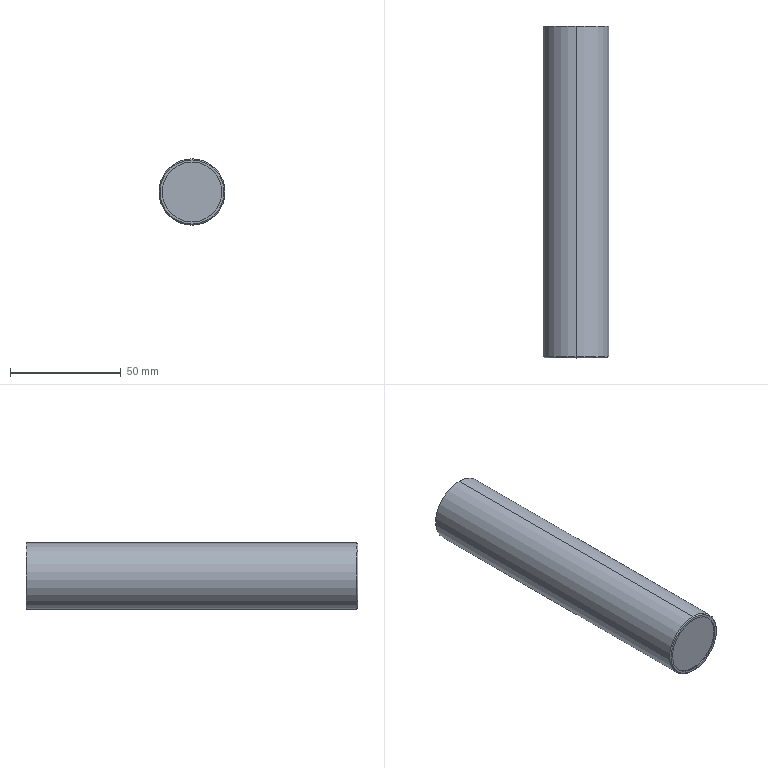Part | SolidWorks | features Chamfer 1, Extrusion 1, RevCut 1 | 1 solid | 12 faces | box 30 x 150 x 30 mm | volume 21279 mm3 | cylinder 6 | plane 4 | cone 2 | commonest cylinder face diameters 27 x4 30 x2
STEP:
#1=CARTESIAN_POINT('',(0.,0.,-14.5));
#2=VERTEX_POINT('',#1);
#3=CARTESIAN_POINT('',(0.,0.,14.5));
#4=VERTEX_POINT('',#3);
#5=CARTESIAN_POINT('',(0.,0.,0.));
#6=DIRECTION('',(0.,-1.,0.));
#7=DIRECTION('',(0.,0.,1.));
#8=AXIS2_PLACEMENT_3D('',#5,#6,#7);
#9=CIRCLE('',#8,14.5);
#10=EDGE_CURVE('',#2,#4,#9,.T.);
#11=ORIENTED_EDGE('',*,*,#10,.F.);
#12=CARTESIAN_POINT('',(0.,0.5,-15.));
#13=VERTEX_POINT('',#12);
#14=CARTESIAN_POINT('',(0.,0.5,-15.));
#15=DIRECTION('',(0.,0.7071,-0.7071));
#16=VECTOR('',#15,1000.);
#17=LINE('',#14,#16);
#18=EDGE_CURVE('',#2,#13,#17,.T.);
#19=ORIENTED_EDGE('',*,*,#18,.T.);
#20=CARTESIAN_POINT('',(0.,0.5,15.));
#21=VERTEX_POINT('',#20);
#22=CARTESIAN_POINT('',(0.,0.5,0.));
#23=DIRECTION('',(0.,1.,0.));
#24=DIRECTION('',(0.,0.,1.));
#25=AXIS2_PLACEMENT_3D('',#22,#23,#24);
#26=CIRCLE('',#25,15.);
#27=EDGE_CURVE('',#21,#13,#26,.T.);
#28=ORIENTED_EDGE('',*,*,#27,.F.);
#29=CARTESIAN_POINT('',(0.,0.5,15.));
#30=DIRECTION('',(0.,0.7071,0.7071));
#31=VECTOR('',#30,1000.);
#32=LINE('',#29,#31);
#33=EDGE_CURVE('',#4,#21,#32,.T.);
#34=ORIENTED_EDGE('',*,*,#33,.F.);
#35=EDGE_LOOP('',(#11,#19,#28,#34));
#36=FACE_OUTER_BOUND('',#35,.T.);
#37=CARTESIAN_POINT('',(0.,0.5,0.));
#38=DIRECTION('',(0.,1.,0.));
#39=DIRECTION('',(0.,0.,1.));
#40=AXIS2_PLACEMENT_3D('',#37,#38,#39);
#41=CONICAL_SURFACE('',#40,15.,0.7854);
#42=ADVANCED_FACE('',(#36),#41,.T.);
#43=CARTESIAN_POINT('',(0.,0.5,13.5));
#44=VERTEX_POINT('',#43);
#45=CARTESIAN_POINT('',(0.,0.5,-13.5));
#46=VERTEX_POINT('',#45);
#47=CARTESIAN_POINT('',(0.,0.5,0.));
#48=DIRECTION('',(0.,-1.,0.));
#49=DIRECTION('',(0.,0.,-1.));
#50=AXIS2_PLACEMENT_3D('',#47,#48,#49);
#51=CIRCLE('',#50,13.5);
#52=EDGE_CURVE('',#44,#46,#51,.T.);
#53=ORIENTED_EDGE('',*,*,#52,.F.);
#54=CARTESIAN_POINT('',(0.,0.,13.5));
#55=VERTEX_POINT('',#54);
#56=CARTESIAN_POINT('',(0.,0.,13.5));
#57=DIRECTION('',(0.,-1.,0.));
#58=VECTOR('',#57,1000.);
#59=LINE('',#56,#58);
#60=EDGE_CURVE('',#44,#55,#59,.T.);
#61=ORIENTED_EDGE('',*,*,#60,.T.);
#62=CARTESIAN_POINT('',(0.,0.,-13.5));
#63=VERTEX_POINT('',#62);
#64=CARTESIAN_POINT('',(0.,0.,0.));
#65=DIRECTION('',(0.,-1.,0.));
#66=DIRECTION('',(0.,0.,-1.));
#67=AXIS2_PLACEMENT_3D('',#64,#65,#66);
#68=CIRCLE('',#67,13.5);
#69=EDGE_CURVE('',#55,#63,#68,.T.);
#70=ORIENTED_EDGE('',*,*,#69,.T.);
#71=CARTESIAN_POINT('',(0.,0.,-13.5));
#72=DIRECTION('',(0.,-1.,0.));
#73=VECTOR('',#72,1000.);
#74=LINE('',#71,#73);
#75=EDGE_CURVE('',#46,#63,#74,.T.);
#76=ORIENTED_EDGE('',*,*,#75,.F.);
#77=EDGE_LOOP('',(#53,#61,#70,#76));
#78=FACE_OUTER_BOUND('',#77,.T.);
#79=CARTESIAN_POINT('',(0.,0.,0.));
#80=DIRECTION('',(0.,-1.,0.));
#81=DIRECTION('',(0.,0.,-1.));
#82=AXIS2_PLACEMENT_3D('',#79,#80,#81);
#83=CYLINDRICAL_SURFACE('',#82,13.5);
#84=ADVANCED_FACE('',(#78),#83,.F.);
#85=CARTESIAN_POINT('',(0.,150.,13.5));
#86=VERTEX_POINT('',#85);
#87=CARTESIAN_POINT('',(0.,150.,-13.5));
#88=VERTEX_POINT('',#87);
#89=CARTESIAN_POINT('',(0.,150.,0.));
#90=DIRECTION('',(0.,-1.,0.));
#91=DIRECTION('',(0.,0.,-1.));
#92=AXIS2_PLACEMENT_3D('',#89,#90,#91);
#93=CIRCLE('',#92,13.5);
#94=EDGE_CURVE('',#86,#88,#93,.T.);
#95=ORIENTED_EDGE('',*,*,#94,.F.);
#96=CARTESIAN_POINT('',(0.,2.5,13.5));
#97=VERTEX_POINT('',#96);
#98=CARTESIAN_POINT('',(0.,0.,13.5));
#99=DIRECTION('',(0.,-1.,0.));
#100=VECTOR('',#99,1000.);
#101=LINE('',#98,#100);
#102=EDGE_CURVE('',#86,#97,#101,.T.);
#103=ORIENTED_EDGE('',*,*,#102,.T.);
#104=CARTESIAN_POINT('',(0.,2.5,-13.5));
#105=VERTEX_POINT('',#104);
#106=CARTESIAN_POINT('',(0.,2.5,0.));
#107=DIRECTION('',(0.,-1.,0.));
#108=DIRECTION('',(0.,0.,-1.));
#109=AXIS2_PLACEMENT_3D('',#106,#107,#108);
#110=CIRCLE('',#109,13.5);
#111=EDGE_CURVE('',#97,#105,#110,.T.);
#112=ORIENTED_EDGE('',*,*,#111,.T.);
#113=CARTESIAN_POINT('',(0.,0.,-13.5));
#114=DIRECTION('',(0.,-1.,0.));
#115=VECTOR('',#114,1000.);
#116=LINE('',#113,#115);
#117=EDGE_CURVE('',#88,#105,#116,.T.);
#118=ORIENTED_EDGE('',*,*,#117,.F.);
#119=EDGE_LOOP('',(#95,#103,#112,#118));
#120=FACE_OUTER_BOUND('',#119,.T.);
#121=CARTESIAN_POINT('',(0.,0.,0.));
#122=DIRECTION('',(0.,-1.,0.));
#123=DIRECTION('',(0.,0.,-1.));
#124=AXIS2_PLACEMENT_3D('',#121,#122,#123);
#125=CYLINDRICAL_SURFACE('',#124,13.5);
#126=ADVANCED_FACE('',(#120),#125,.F.);
#127=CARTESIAN_POINT('',(0.,150.,15.));
#128=VERTEX_POINT('',#127);
#129=CARTESIAN_POINT('',(0.,150.,-15.));
#130=VERTEX_POINT('',#129);
#131=CARTESIAN_POINT('',(0.,150.,0.));
#132=DIRECTION('',(0.,1.,0.));
#133=DIRECTION('',(0.,0.,1.));
#134=AXIS2_PLACEMENT_3D('',#131,#132,#133);
#135=CIRCLE('',#134,15.);
#136=EDGE_CURVE('',#128,#130,#135,.T.);
#137=ORIENTED_EDGE('',*,*,#136,.F.);
#138=CARTESIAN_POINT('',(0.,150.,15.));
#139=DIRECTION('',(0.,-1.,0.));
#140=VECTOR('',#139,1000.);
#141=LINE('',#138,#140);
#142=EDGE_CURVE('',#128,#21,#141,.T.);
#143=ORIENTED_EDGE('',*,*,#142,.T.);
#144=ORIENTED_EDGE('',*,*,#27,.T.);
#145=CARTESIAN_POINT('',(0.,150.,-15.));
#146=DIRECTION('',(0.,-1.,0.));
#147=VECTOR('',#146,1000.);
#148=LINE('',#145,#147);
#149=EDGE_CURVE('',#130,#13,#148,.T.);
#150=ORIENTED_EDGE('',*,*,#149,.F.);
#151=EDGE_LOOP('',(#137,#143,#144,#150));
#152=FACE_OUTER_BOUND('',#151,.T.);
#153=CARTESIAN_POINT('',(0.,150.,0.));
#154=DIRECTION('',(0.,-1.,0.));
#155=DIRECTION('',(0.,0.,-1.));
#156=AXIS2_PLACEMENT_3D('',#153,#154,#155);
#157=CYLINDRICAL_SURFACE('',#156,15.);
#158=ADVANCED_FACE('',(#152),#157,.T.);
#159=ORIENTED_EDGE('',*,*,#142,.F.);
#160=CARTESIAN_POINT('',(0.,150.,0.));
#161=DIRECTION('',(0.,1.,0.));
#162=DIRECTION('',(0.,0.,1.));
#163=AXIS2_PLACEMENT_3D('',#160,#161,#162);
#164=CIRCLE('',#163,15.);
#165=EDGE_CURVE('',#130,#128,#164,.T.);
#166=ORIENTED_EDGE('',*,*,#165,.F.);
#167=ORIENTED_EDGE('',*,*,#149,.T.);
#168=CARTESIAN_POINT('',(0.,0.5,0.));
#169=DIRECTION('',(0.,1.,0.));
#170=DIRECTION('',(0.,0.,1.));
#171=AXIS2_PLACEMENT_3D('',#168,#169,#170);
#172=CIRCLE('',#171,15.);
#173=EDGE_CURVE('',#13,#21,#172,.T.);
#174=ORIENTED_EDGE('',*,*,#173,.T.);
#175=EDGE_LOOP('',(#159,#166,#167,#174));
#176=FACE_OUTER_BOUND('',#175,.T.);
#177=CARTESIAN_POINT('',(0.,150.,0.));
#178=DIRECTION('',(0.,-1.,0.));
#179=DIRECTION('',(0.,0.,-1.));
#180=AXIS2_PLACEMENT_3D('',#177,#178,#179);
#181=CYLINDRICAL_SURFACE('',#180,15.);
#182=ADVANCED_FACE('',(#176),#181,.T.);
#183=CARTESIAN_POINT('',(0.,150.,0.));
#184=DIRECTION('',(0.,-1.,0.));
#185=DIRECTION('',(0.,0.,-1.));
#186=AXIS2_PLACEMENT_3D('',#183,#184,#185);
#187=CIRCLE('',#186,13.5);
#188=EDGE_CURVE('',#88,#86,#187,.T.);
#189=ORIENTED_EDGE('',*,*,#188,.T.);
#190=ORIENTED_EDGE('',*,*,#94,.T.);
#191=EDGE_LOOP('',(#189,#190));
#192=FACE_BOUND('',#191,.T.);
#193=ORIENTED_EDGE('',*,*,#165,.T.);
#194=ORIENTED_EDGE('',*,*,#136,.T.);
#195=EDGE_LOOP('',(#193,#194));
#196=FACE_OUTER_BOUND('',#195,.T.);
#197=CARTESIAN_POINT('',(0.,150.,0.));
#198=DIRECTION('',(0.,1.,0.));
#199=DIRECTION('',(0.,0.,1.));
#200=AXIS2_PLACEMENT_3D('',#197,#198,#199);
#201=PLANE('',#200);
#202=ADVANCED_FACE('',(#192,#196),#201,.T.);
#203=CARTESIAN_POINT('',(0.,0.,0.));
#204=DIRECTION('',(0.,-1.,0.));
#205=DIRECTION('',(0.,0.,1.));
#206=AXIS2_PLACEMENT_3D('',#203,#204,#205);
#207=CIRCLE('',#206,14.5);
#208=EDGE_CURVE('',#4,#2,#207,.T.);
#209=ORIENTED_EDGE('',*,*,#208,.T.);
#210=ORIENTED_EDGE('',*,*,#10,.T.);
#211=EDGE_LOOP('',(#209,#210));
#212=FACE_OUTER_BOUND('',#211,.T.);
#213=CARTESIAN_POINT('',(0.,0.,0.));
#214=DIRECTION('',(0.,-1.,0.));
#215=DIRECTION('',(0.,0.,-1.));
#216=AXIS2_PLACEMENT_3D('',#213,#214,#215);
#217=CIRCLE('',#216,13.5);
#218=EDGE_CURVE('',#63,#55,#217,.T.);
#219=ORIENTED_EDGE('',*,*,#218,.F.);
#220=ORIENTED_EDGE('',*,*,#69,.F.);
#221=EDGE_LOOP('',(#219,#220));
#222=FACE_BOUND('',#221,.T.);
#223=CARTESIAN_POINT('',(0.,0.,0.));
#224=DIRECTION('',(0.,1.,0.));
#225=DIRECTION('',(0.,0.,1.));
#226=AXIS2_PLACEMENT_3D('',#223,#224,#225);
#227=PLANE('',#226);
#228=ADVANCED_FACE('',(#212,#222),#227,.F.);
#229=CARTESIAN_POINT('',(0.,2.5,0.));
#230=DIRECTION('',(0.,-1.,0.));
#231=DIRECTION('',(0.,0.,-1.));
#232=AXIS2_PLACEMENT_3D('',#229,#230,#231);
#233=CIRCLE('',#232,13.5);
#234=EDGE_CURVE('',#105,#97,#233,.T.);
#235=ORIENTED_EDGE('',*,*,#234,.F.);
#236=ORIENTED_EDGE('',*,*,#111,.F.);
#237=EDGE_LOOP('',(#235,#236));
#238=FACE_OUTER_BOUND('',#237,.T.);
#239=CARTESIAN_POINT('',(0.,2.5,0.));
#240=DIRECTION('',(0.,-1.,0.));
#241=DIRECTION('',(0.,0.,-1.));
#242=AXIS2_PLACEMENT_3D('',#239,#240,#241);
#243=PLANE('',#242);
#244=ADVANCED_FACE('',(#238),#243,.F.);
#245=ORIENTED_EDGE('',*,*,#102,.F.);
#246=ORIENTED_EDGE('',*,*,#188,.F.);
#247=ORIENTED_EDGE('',*,*,#117,.T.);
#248=ORIENTED_EDGE('',*,*,#234,.T.);
#249=EDGE_LOOP('',(#245,#246,#247,#248));
#250=FACE_OUTER_BOUND('',#249,.T.);
#251=CARTESIAN_POINT('',(0.,0.,0.));
#252=DIRECTION('',(0.,-1.,0.));
#253=DIRECTION('',(0.,0.,-1.));
#254=AXIS2_PLACEMENT_3D('',#251,#252,#253);
#255=CYLINDRICAL_SURFACE('',#254,13.5);
#256=ADVANCED_FACE('',(#250),#255,.F.);
#257=CARTESIAN_POINT('',(0.,0.5,0.));
#258=DIRECTION('',(0.,-1.,0.));
#259=DIRECTION('',(0.,0.,-1.));
#260=AXIS2_PLACEMENT_3D('',#257,#258,#259);
#261=CIRCLE('',#260,13.5);
#262=EDGE_CURVE('',#46,#44,#261,.T.);
#263=ORIENTED_EDGE('',*,*,#262,.T.);
#264=ORIENTED_EDGE('',*,*,#52,.T.);
#265=EDGE_LOOP('',(#263,#264));
#266=FACE_OUTER_BOUND('',#265,.T.);
#267=CARTESIAN_POINT('',(0.,0.5,0.));
#268=DIRECTION('',(0.,1.,0.));
#269=DIRECTION('',(0.,0.,1.));
#270=AXIS2_PLACEMENT_3D('',#267,#268,#269);
#271=PLANE('',#270);
#272=ADVANCED_FACE('',(#266),#271,.F.);
#273=ORIENTED_EDGE('',*,*,#60,.F.);
#274=ORIENTED_EDGE('',*,*,#262,.F.);
#275=ORIENTED_EDGE('',*,*,#75,.T.);
#276=ORIENTED_EDGE('',*,*,#218,.T.);
#277=EDGE_LOOP('',(#273,#274,#275,#276));
#278=FACE_OUTER_BOUND('',#277,.T.);
#279=CARTESIAN_POINT('',(0.,0.,0.));
#280=DIRECTION('',(0.,-1.,0.));
#281=DIRECTION('',(0.,0.,-1.));
#282=AXIS2_PLACEMENT_3D('',#279,#280,#281);
#283=CYLINDRICAL_SURFACE('',#282,13.5);
#284=ADVANCED_FACE('',(#278),#283,.F.);
#285=ORIENTED_EDGE('',*,*,#18,.F.);
#286=ORIENTED_EDGE('',*,*,#208,.F.);
#287=ORIENTED_EDGE('',*,*,#33,.T.);
#288=ORIENTED_EDGE('',*,*,#173,.F.);
#289=EDGE_LOOP('',(#285,#286,#287,#288));
#290=FACE_OUTER_BOUND('',#289,.T.);
#291=CARTESIAN_POINT('',(0.,0.5,0.));
#292=DIRECTION('',(0.,1.,0.));
#293=DIRECTION('',(0.,0.,1.));
#294=AXIS2_PLACEMENT_3D('',#291,#292,#293);
#295=CONICAL_SURFACE('',#294,15.,0.7854);
#296=ADVANCED_FACE('',(#290),#295,.T.);
#297=CLOSED_SHELL('',(#42,#84,#126,#158,#182,#202,#228,#244,#256,#272,#284,#296));
#298=MANIFOLD_SOLID_BREP('',#297);
#299=CARTESIAN_POINT('',(0.,0.,0.));
#300=DIRECTION('',(0.,0.,1.));
#301=DIRECTION('',(1.,0.,0.));
#302=AXIS2_PLACEMENT_3D('',#299,#300,#301);
#303=(LENGTH_UNIT()NAMED_UNIT(*)SI_UNIT(.MILLI.,.METRE.));
#304=UNCERTAINTY_MEASURE_WITH_UNIT(LENGTH_MEASURE(0.00001),#303,'','');
#305=(NAMED_UNIT(*)PLANE_ANGLE_UNIT()SI_UNIT($,.RADIAN.));
#306=(NAMED_UNIT(*)SI_UNIT($,.STERADIAN.)SOLID_ANGLE_UNIT());
#307=(GEOMETRIC_REPRESENTATION_CONTEXT(3)GLOBAL_UNCERTAINTY_ASSIGNED_CONTEXT((#304))GLOBAL_UNIT_ASSIGNED_CONTEXT((#303,#305,#306))REPRESENTATION_CONTEXT('',''));
#308=ADVANCED_BREP_SHAPE_REPRESENTATION('',(#298,#302),#307);